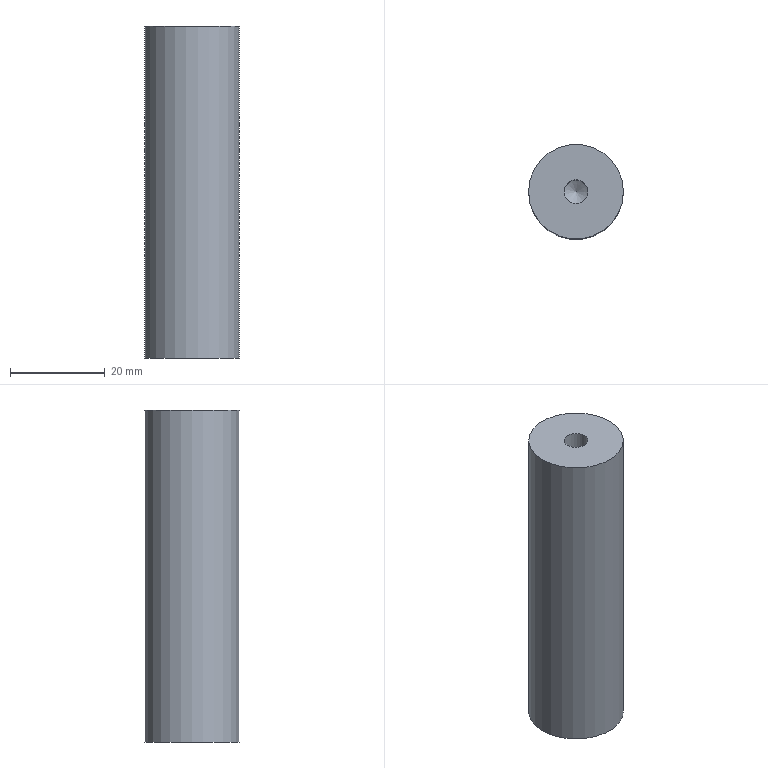Part | NX | features LIN_SOLID_COLOR 2 | 1 solid | 5 faces | box 20 x 20 x 70 mm | volume 21588 mm3 | plane 2 | cylinder 2 | cone 1 | commonest cylinder face diameters 5.006 x1 20 x1
STEP:
#1=CARTESIAN_POINT('',(668.381,-22.569,140.));
#2=VERTEX_POINT('',#1);
#3=CARTESIAN_POINT('',(665.878,-22.569,140.));
#4=DIRECTION('',(0.,0.,1.));
#5=DIRECTION('',(1.,0.,0.));
#6=AXIS2_PLACEMENT_3D('',#3,#4,#5);
#7=CIRCLE('',#6,2.503);
#8=EDGE_CURVE('',#2,#2,#7,.T.);
#9=ORIENTED_EDGE('',*,*,#8,.F.);
#10=EDGE_LOOP('',(#9));
#11=FACE_BOUND('',#10,.T.);
#12=CARTESIAN_POINT('',(675.878,-22.569,140.));
#13=VERTEX_POINT('',#12);
#14=CARTESIAN_POINT('',(665.878,-22.569,140.));
#15=DIRECTION('',(0.,0.,1.));
#16=DIRECTION('',(1.,0.,0.));
#17=AXIS2_PLACEMENT_3D('',#14,#15,#16);
#18=CIRCLE('',#17,10.);
#19=EDGE_CURVE('',#13,#13,#18,.T.);
#20=ORIENTED_EDGE('',*,*,#19,.T.);
#21=EDGE_LOOP('',(#20));
#22=FACE_BOUND('',#21,.T.);
#23=CARTESIAN_POINT('',(1237.878,-22.569,140.));
#24=DIRECTION('',(0.,0.,1.));
#25=DIRECTION('',(1.,0.,0.));
#26=AXIS2_PLACEMENT_3D('',#23,#24,#25);
#27=PLANE('',#26);
#28=ADVANCED_FACE('',(#11,#22),#27,.T.);
#29=ORIENTED_EDGE('',*,*,#19,.F.);
#30=EDGE_LOOP('',(#29));
#31=FACE_BOUND('',#30,.T.);
#32=CARTESIAN_POINT('',(675.878,-22.569,70.));
#33=VERTEX_POINT('',#32);
#34=CARTESIAN_POINT('',(665.878,-22.569,70.));
#35=DIRECTION('',(0.,0.,1.));
#36=DIRECTION('',(1.,0.,0.));
#37=AXIS2_PLACEMENT_3D('',#34,#35,#36);
#38=CIRCLE('',#37,10.);
#39=EDGE_CURVE('',#33,#33,#38,.T.);
#40=ORIENTED_EDGE('',*,*,#39,.T.);
#41=EDGE_LOOP('',(#40));
#42=FACE_BOUND('',#41,.T.);
#43=CARTESIAN_POINT('',(665.878,-22.569,305.));
#44=DIRECTION('',(0.,0.,-1.));
#45=DIRECTION('',(-1.,0.,0.));
#46=AXIS2_PLACEMENT_3D('',#43,#44,#45);
#47=CYLINDRICAL_SURFACE('',#46,10.);
#48=ADVANCED_FACE('',(#31,#42),#47,.T.);
#49=ORIENTED_EDGE('',*,*,#39,.F.);
#50=EDGE_LOOP('',(#49));
#51=FACE_BOUND('',#50,.T.);
#52=CARTESIAN_POINT('',(658.728,-34.001,70.));
#53=DIRECTION('',(0.,0.,1.));
#54=DIRECTION('',(1.,0.,0.));
#55=AXIS2_PLACEMENT_3D('',#52,#53,#54);
#56=PLANE('',#55);
#57=ADVANCED_FACE('',(#51),#56,.F.);
#58=CARTESIAN_POINT('',(668.381,-22.569,120.));
#59=VERTEX_POINT('',#58);
#60=CARTESIAN_POINT('',(665.878,-22.569,120.));
#61=DIRECTION('',(0.,0.,-1.));
#62=DIRECTION('',(1.,0.,0.));
#63=AXIS2_PLACEMENT_3D('',#60,#61,#62);
#64=CIRCLE('',#63,2.503);
#65=EDGE_CURVE('',#59,#59,#64,.F.);
#66=ORIENTED_EDGE('',*,*,#65,.T.);
#67=EDGE_LOOP('',(#66));
#68=FACE_BOUND('',#67,.T.);
#69=CARTESIAN_POINT('',(665.878,-22.569,118.555));
#70=VERTEX_POINT('',#69);
#71=VERTEX_LOOP('',#70);
#72=FACE_BOUND('',#71,.T.);
#73=CARTESIAN_POINT('',(665.878,-22.569,118.555));
#74=DIRECTION('',(0.,0.,1.));
#75=DIRECTION('',(1.,0.,0.));
#76=AXIS2_PLACEMENT_3D('',#73,#74,#75);
#77=CONICAL_SURFACE('',#76,0.,1.047);
#78=ADVANCED_FACE('',(#68,#72),#77,.F.);
#79=ORIENTED_EDGE('',*,*,#65,.F.);
#80=EDGE_LOOP('',(#79));
#81=FACE_BOUND('',#80,.T.);
#82=ORIENTED_EDGE('',*,*,#8,.T.);
#83=EDGE_LOOP('',(#82));
#84=FACE_BOUND('',#83,.T.);
#85=CARTESIAN_POINT('',(665.878,-22.569,135.));
#86=DIRECTION('',(0.,0.,-1.));
#87=DIRECTION('',(1.,0.,0.));
#88=AXIS2_PLACEMENT_3D('',#85,#86,#87);
#89=CYLINDRICAL_SURFACE('',#88,2.503);
#90=ADVANCED_FACE('',(#81,#84),#89,.F.);
#91=CLOSED_SHELL('',(#28,#48,#57,#78,#90));
#92=MANIFOLD_SOLID_BREP('',#91);
#93=(LENGTH_UNIT()NAMED_UNIT(*)SI_UNIT(.MILLI.,.METRE.));
#94=UNCERTAINTY_MEASURE_WITH_UNIT(LENGTH_MEASURE(0.00001),#93,'','');
#95=(NAMED_UNIT(*)PLANE_ANGLE_UNIT()SI_UNIT($,.RADIAN.));
#96=(NAMED_UNIT(*)SI_UNIT($,.STERADIAN.)SOLID_ANGLE_UNIT());
#97=(GEOMETRIC_REPRESENTATION_CONTEXT(3)GLOBAL_UNCERTAINTY_ASSIGNED_CONTEXT((#94))GLOBAL_UNIT_ASSIGNED_CONTEXT((#93,#95,#96))REPRESENTATION_CONTEXT('',''));
#98=ADVANCED_BREP_SHAPE_REPRESENTATION('',(#92),#97);